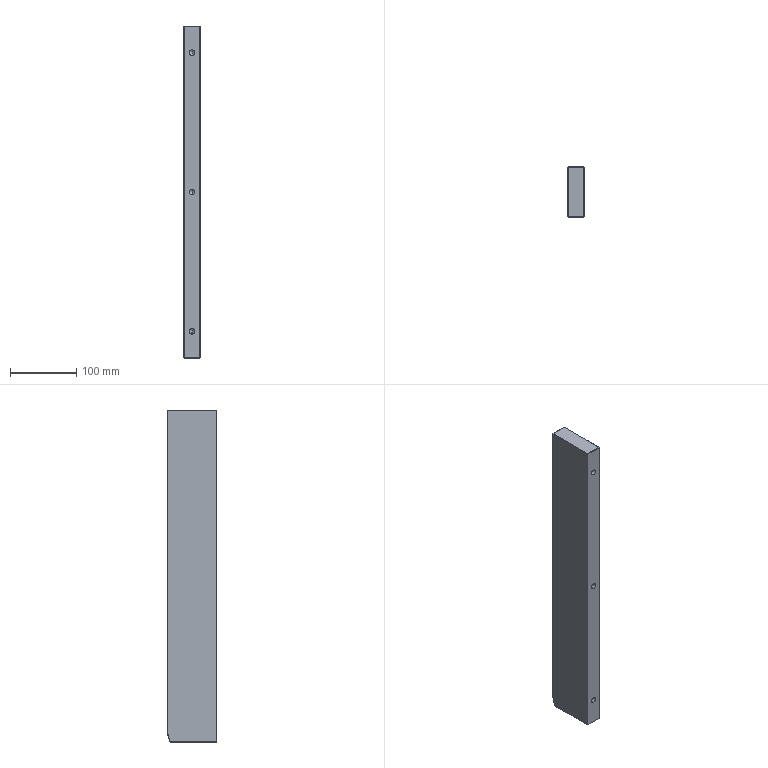Part | STEP file | OP10-018_base rib (A) | 1 solid | 45 faces | box 25 x 75 x 500 mm | volume 930693 mm3 | plane 29 | cylinder 8 | cone 8 | commonest cylinder face diameters 8.5 x8